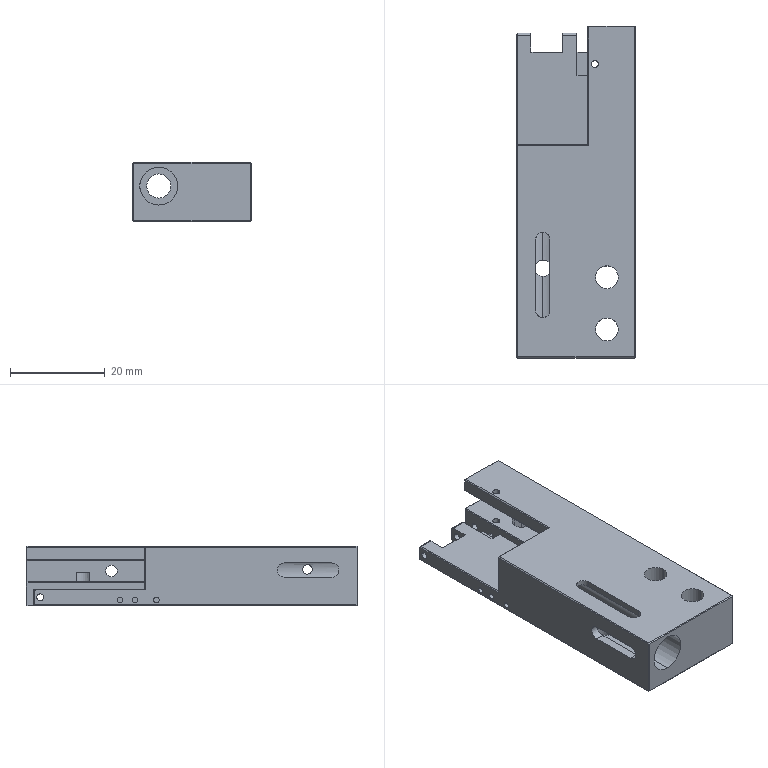Part | SolidWorks | features Cut 13, ICE 4, Chamfer 3, Fillet 2, 3DProfileFeature 1, Extrusion 1, HoleWzd 1 | 1 solid | 121 faces | box 25 x 70 x 12.5 mm | volume 14176 mm3 | plane 69 | cylinder 47 | cone 5 | commonest cylinder face diameters 1.5 x13 1.2 x6 8 x6 3 x5 4.8 x4 4 x3